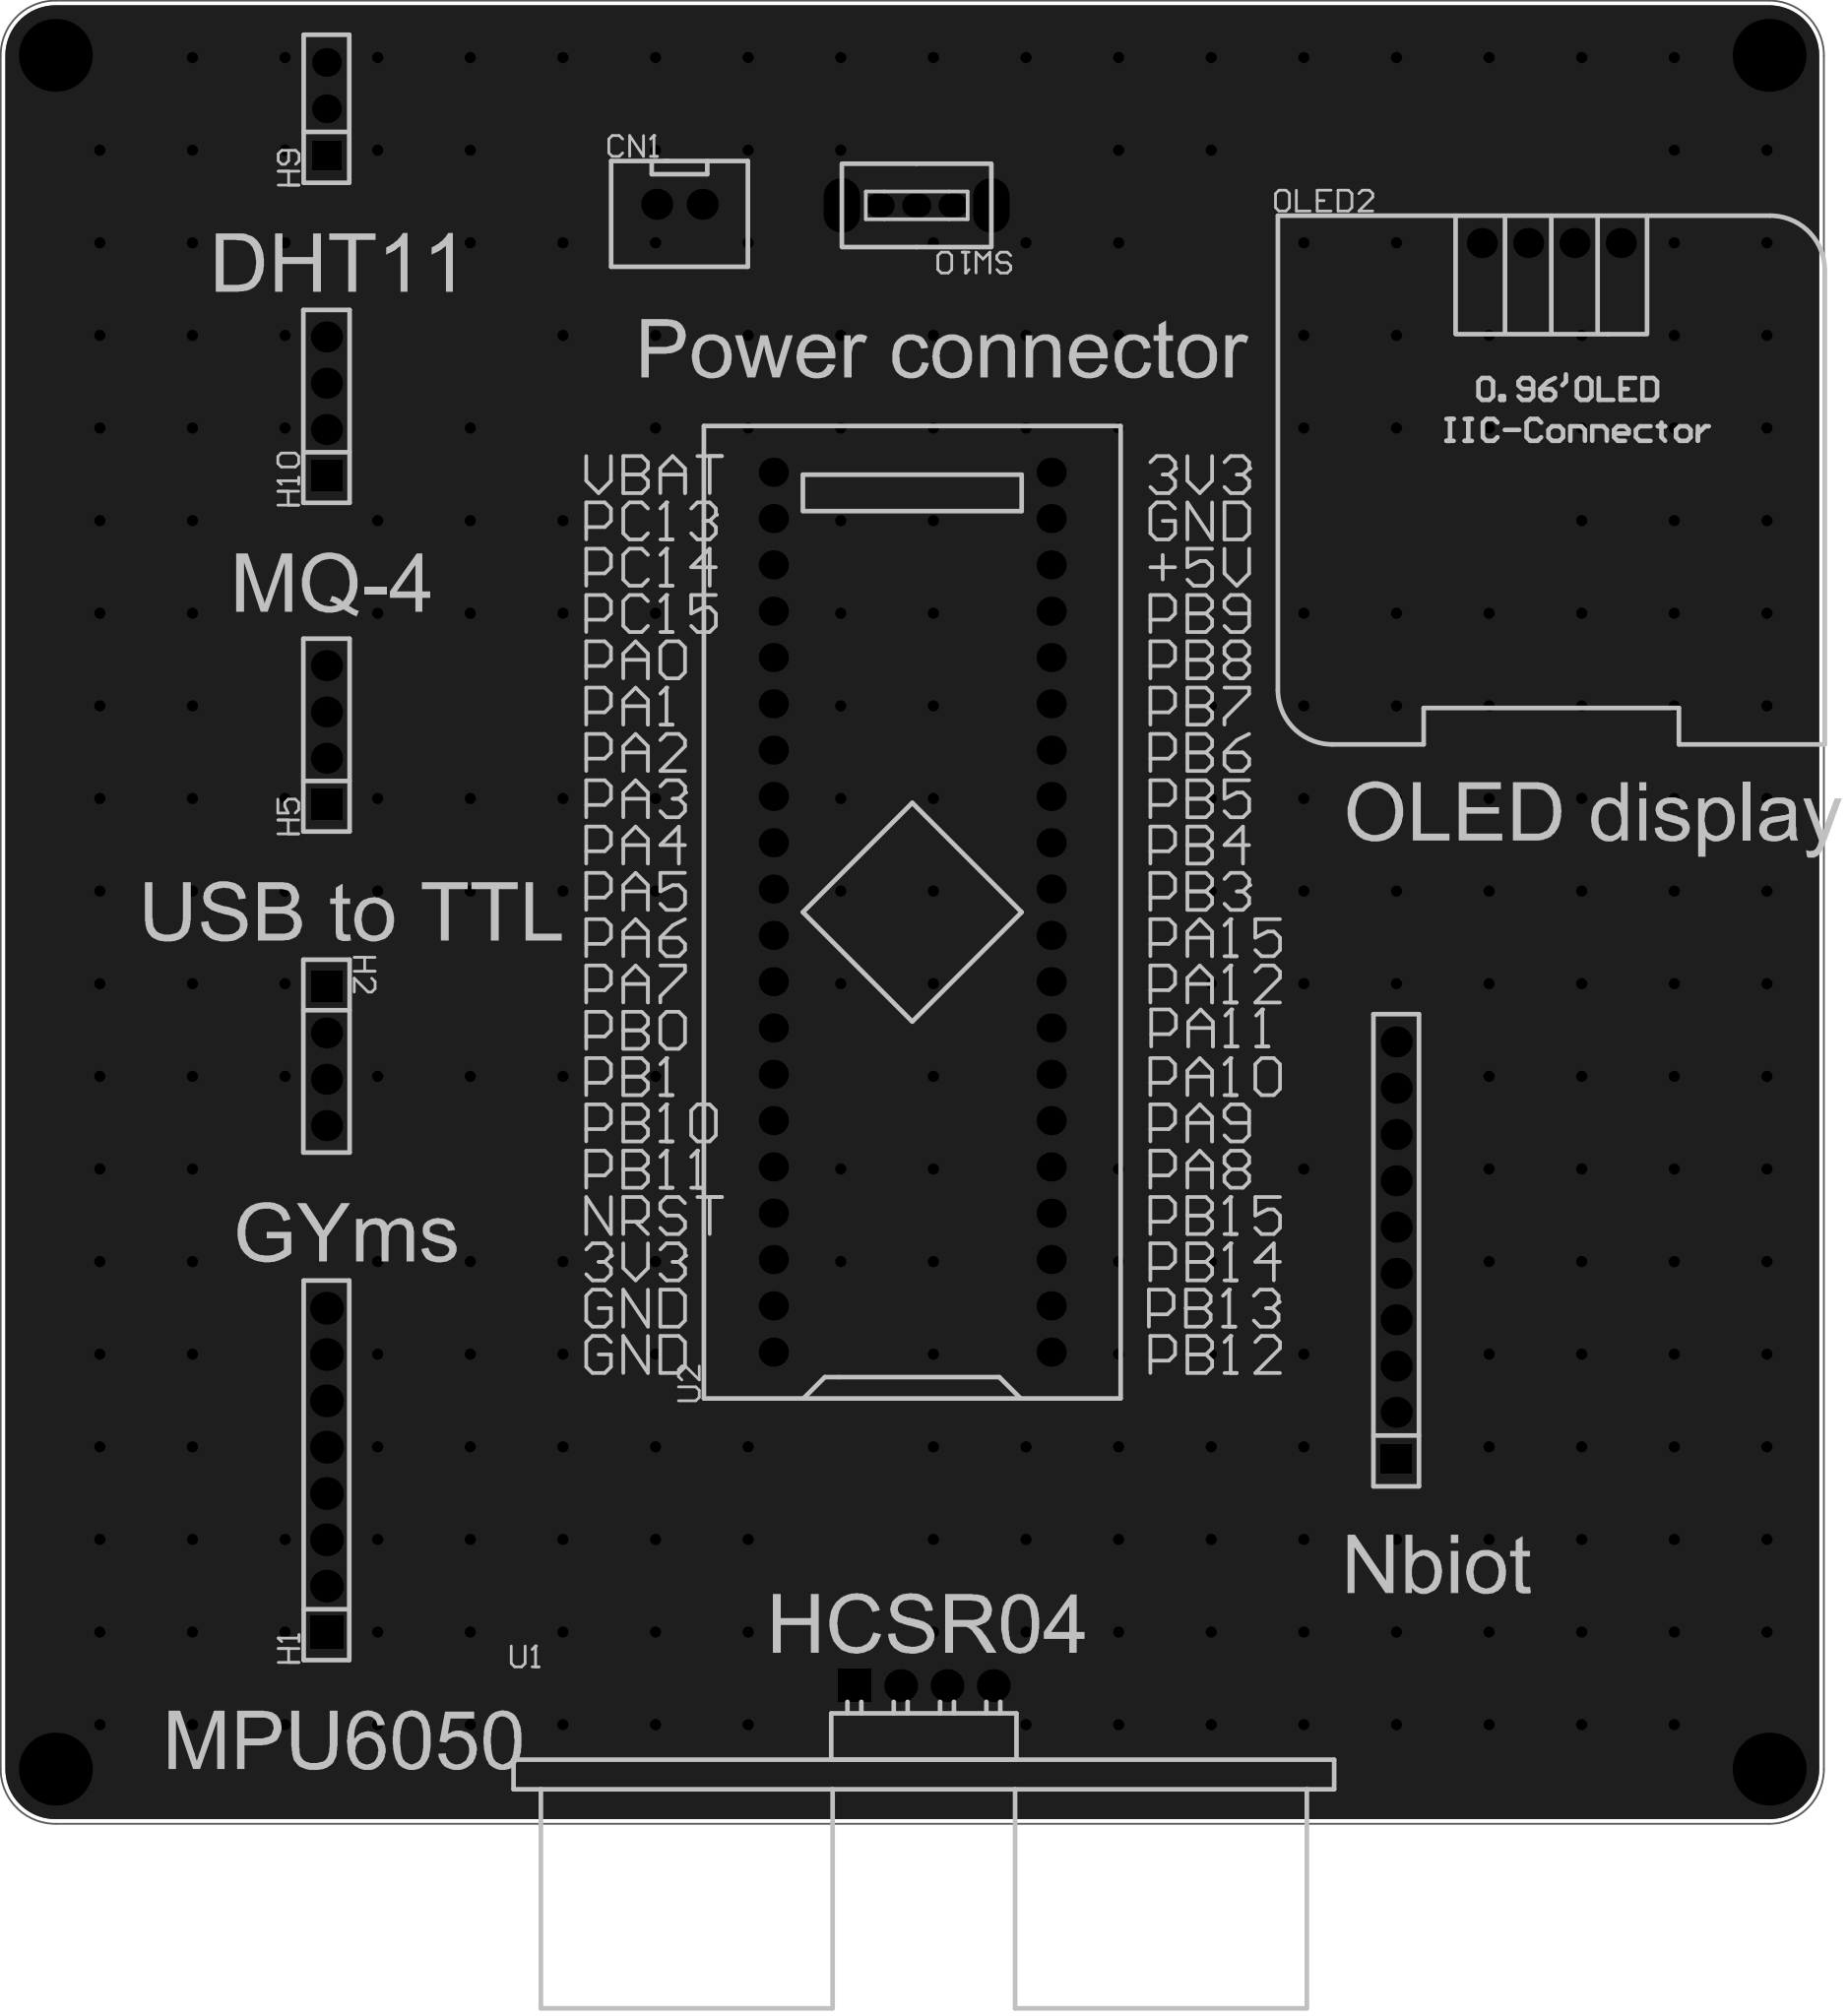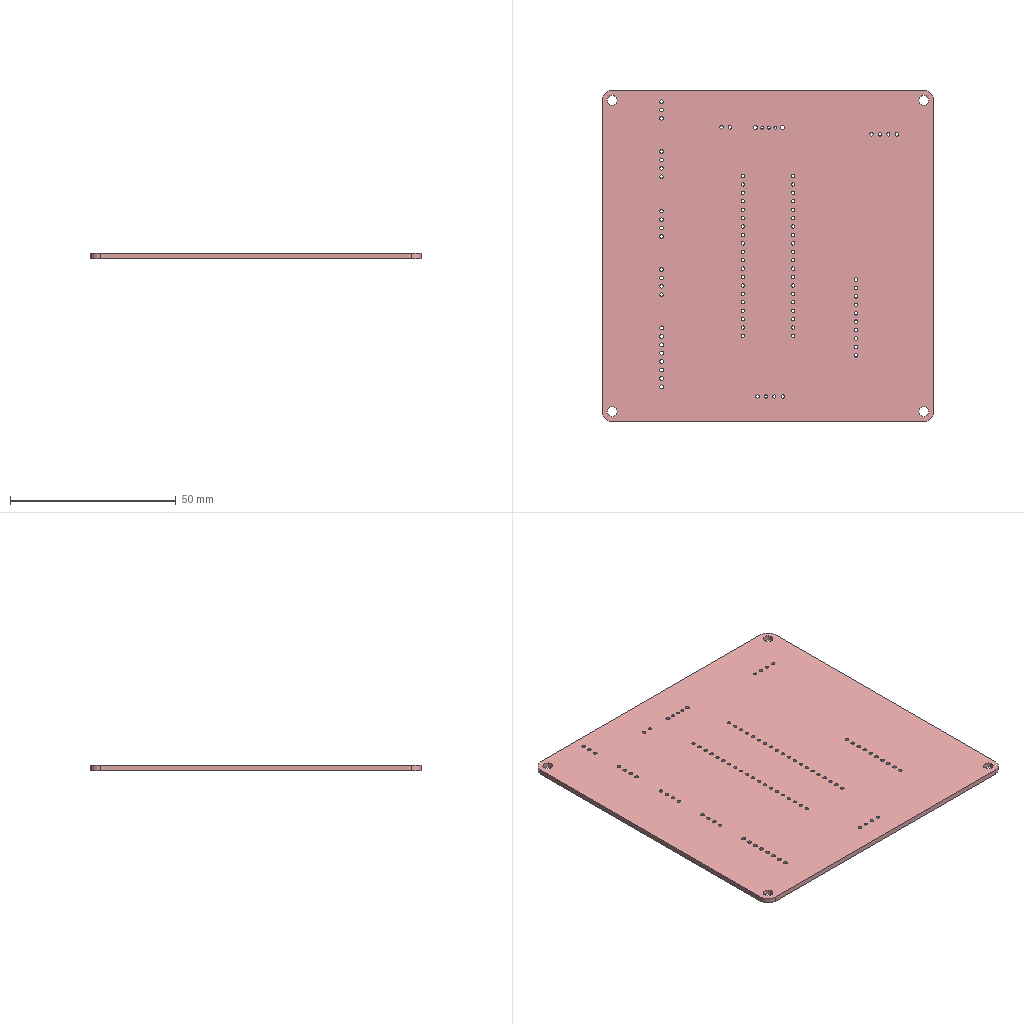Circuit board layout | Altium Designer | box 100 x 100 x 1.6 mm
Layer stack:
# Altium Designer layer stack of  (unit mm; dielectric type: 0 none, 1 core, 2 prepreg, 3 surface material)
index,name,kind,layer,copper_thickness_mm,dielectric_type,dielectric_thickness_mm,dielectric_material,dielectric_constant
0,Top Paste Mask Layer,other,,,,,,
1,Top Silkscreen Layer,other,,,,,,
2,Top Solder Mask Layer,dielectric,,,3,0.01,,3.3
3,Top Layer,copper,Top Layer,0.035,,,,
4,Dielectric1,dielectric,,,3,1.51,FR4,4.5
5,Bottom Layer,copper,Bottom Layer,0.035,,,,
6,Bottom Solder Mask Layer,dielectric,,,3,0.01,,3.3
7,Bottom Silkscreen Layer,other,,,,,,
8,Bottom Paste Mask Layer,other,,,,,,
# drill layer pairs: low layer,high layer
drill_pair,Top Layer,Bottom Layer
Part placement:
Designator,Comment,Layer,Footprint,Center-X(mm),Center-Y(mm),Rotation
CN1,XH2.54*2P_straight,TopLayer,CONN-TH_2P-P2.50-XH2.54-2P,128.583,175.206,0
H1,,TopLayer,HDR-TH_8P-P2.54-V-F-1,109.22,105.766,90
H2,,TopLayer,HDR-TH_4P-P2.54-V-F,109.22,128.485,270
H5,,TopLayer,HDR-TH_4P-P2.54-V-F,109.22,146.092,90
H9,,TopLayer,HDR-TH_3P-P2.54-V-F,109.22,180.447,90
H10,,TopLayer,HDR-TH_4P-P2.54-V-F,109.22,164.123,90
OLED2,,TopLayer,0.96OLED_4P,176.403,173.081,0
SW10,,TopLayer,拨动开关,141.588,175.147,180
H6,,TopLayer,HDR-TH_10P-P2.54-V-F,167.894,117.836,90
U1,HC-SR04,TopLayer,TH_HC-SR04V,141.986,93.96,0
U2,STM32F103C8T6-Card,TopLayer,CONN-TH_L53.3-W22.9_STM32F103C8T6-CARD,141.351,136.378,90
Pad and via stacks:
# Altium Designer via and pad stacks of  (unit mm). Each distinct definition once, with the count of objects using it.
# via: kind,start_layer,end_layer,hole_mm,diameter_mm,mode(0 simple;1 top-mid-bottom;2 full stack),diameter_per_layer,count,example_net
# pad: kind,layer,hole_mm,hole_type(0 round;1 square;2 slot),plating,top_size,top_shape(1 round;2 rect;3 octagon;9 rounded rect),mid_size,bottom_size,mode,footprint,size_per_layer,count,example
pad,Multi-Layer,3,0,plated,4x4,1,4x4,4x4,0,,,4,1
pad,Multi-Layer,1.05,0,plated,1.7x1.7,1,1.7x1.7,1.7x1.7,0,CONN-TH_2P-P2.50-XH2.54-2P,,2,CN1.2
pad,Multi-Layer,1.2,0,plated,1.8x1.8,2,1.8x1.8,1.8x1.8,0,HDR-TH_8P-P2.54-V-F-1,,1,H1.1
pad,Multi-Layer,1.2,0,plated,1.8x1.8,1,1.8x1.8,1.8x1.8,0,HDR-TH_8P-P2.54-V-F-1,,7,H1.2
pad,Multi-Layer,1.1,0,plated,1.7x1.7,2,1.7x1.7,1.7x1.7,0,HDR-TH_4P-P2.54-V-F,,3,H2.1
pad,Multi-Layer,1.1,0,plated,1.7x1.7,1,1.7x1.7,1.7x1.7,0,HDR-TH_4P-P2.54-V-F,,9,H2.2
pad,Multi-Layer,1.02,0,plated,1.575x1.575,1,1.575x1.575,1.575x1.575,0,HDR-TH_3P-P2.54-V-F,,2,H9.3
pad,Multi-Layer,1.02,0,plated,1.575x1.575,2,1.575x1.575,1.575x1.575,0,HDR-TH_3P-P2.54-V-F,,1,H9.1
pad,Multi-Layer,1,0,plated,1.65x1.65,1,1.65x1.65,1.65x1.65,0,0.96OLED_4P,,4,OLED2.4
pad,Multi-Layer,0.8992,0,plated,1.6x1.3,1,1.6x1.3,1.6x1.3,0,\u00B2\u00A6\u00B6\u00AF\u00BF\u00AA\u00B9\u00D8,,3,SW10.1
pad,Multi-Layer,1.3,0,plated,3x1.999,1,3x1.999,3x1.999,0,\u00B2\u00A6\u00B6\u00AF\u00BF\u00AA\u00B9\u00D8,,2,SW10.4
pad,Multi-Layer,1.1,0,plated,1.7x1.7,1,1.7x1.7,1.7x1.7,0,HDR-TH_10P-P2.54-V-F,,9,H6.10
pad,Multi-Layer,1.1,0,plated,1.575x1.7,2,1.575x1.7,1.575x1.7,0,HDR-TH_10P-P2.54-V-F,,1,H6.1
pad,Multi-Layer,1.001,0,plated,1.8x1.8,1,1.8x1.8,1.8x1.8,0,TH_HC-SR04V,,3,U1.4
pad,Multi-Layer,1.001,0,plated,1.8x1.8,2,1.8x1.8,1.8x1.8,0,TH_HC-SR04V,,1,U1.1
pad,Multi-Layer,1,0,plated,1.6x1.6,1,1.6x1.6,1.6x1.6,0,CONN-TH_L53.3-W22.9_STM32F103C8T6-CARD,,40,U2.1
via,Top Layer,Bottom Layer,0.3048,0.61,0,,272,GND
Copper pours:
name,layer,net,type(0 solid;1 hatched;2 none)
Bottom Layer-GND,Bottom Layer,GND,0
Top Layer-GND,Top Layer,GND,0
Design rules, without the lines most boards share:
# Altium Designer design rules of  (exported by Altium Designer, unit mm)
# columns: name | kind | enabled | priority | scope1 | scope2 | descriptor | typed fields (field=value)
Copper_copperRegion_copperThickness1oz | 0 | disabled | 4 | All | All | Clearance Constraint (Gap=5.984mil) (Disabled)(All),(All) | gap=0.152
Copper_copperRegion_copperThickness1oz_1 | 63 | disabled | 4 | All | All | Board Clearance Constraint (Gap=0mil) (Disabled)(All) |
Copper_copperRegion_Copper_copperRegion | 0 | disabled | 5 | All | All | Clearance Constraint (Gap=5.984mil) (Disabled)(All),(All) | gap=0.152
Copper_copperRegion_Copper_copperRegion_1 | 63 | disabled | 5 | All | All | Board Clearance Constraint (Gap=0mil) (Disabled)(All) |
copperThickness1oz | 0 | enabled | 6 | All | All | Clearance Constraint (Gap=5.984mil) (All),(All) | gap=0.152
copperThickness1oz_1 | 63 | enabled | 6 | All | All | Board Clearance Constraint (Gap=0mil) (All) |
copperRegion_copperThickness1oz | 20 | disabled | 1 | All | All | Polygon Connect Rule(Relief Connect )(Conductor Width=10mil) (Relief Angle=90 Angle) (Entries=4) (Air Gap Width=10mil) (Disabled)(All),(All) | connect_style(0=relief,1=direct,2=none)=0 relief_conductor_width=0.254 relief_entries=4
copperRegion_Copper_copperRegion | 20 | disabled | 2 | All | All | Polygon Connect Rule(Relief Connect )(Conductor Width=10mil) (Relief Angle=90 Angle) (Entries=4) (Air Gap Width=10mil) (Disabled)(All),(All) | connect_style(0=relief,1=direct,2=none)=0 relief_conductor_width=0.254 relief_entries=4
copperRegion | 20 | enabled | 3 | All | All | Polygon Connect Rule(Relief Connect )(Conductor Width=10mil) (Relief Angle=90 Angle) (Entries=4) (Air Gap Width=10mil) (All),(All) | connect_style(0=relief,1=direct,2=none)=0 relief_conductor_width=0.254 relief_entries=4